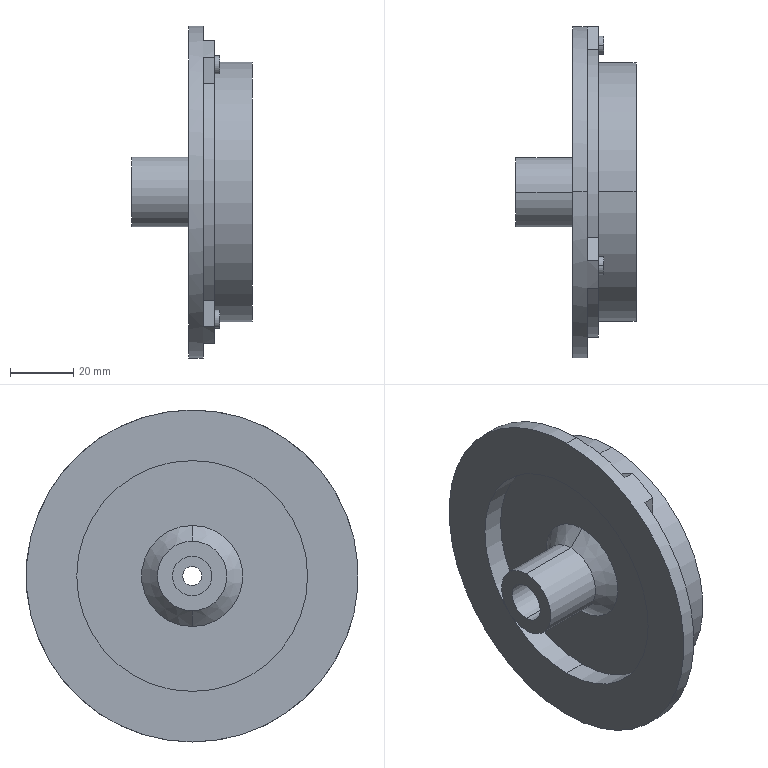Part | STEP file | Mkt hub | 1 solid | 50 faces | box 38 x 105 x 105 mm | volume 81740 mm3 | cylinder 26 | plane 20 | cone 4 | commonest cylinder face diameters 5.8 x6 92 x4 6 x2 12.5 x2 17 x2 22 x2